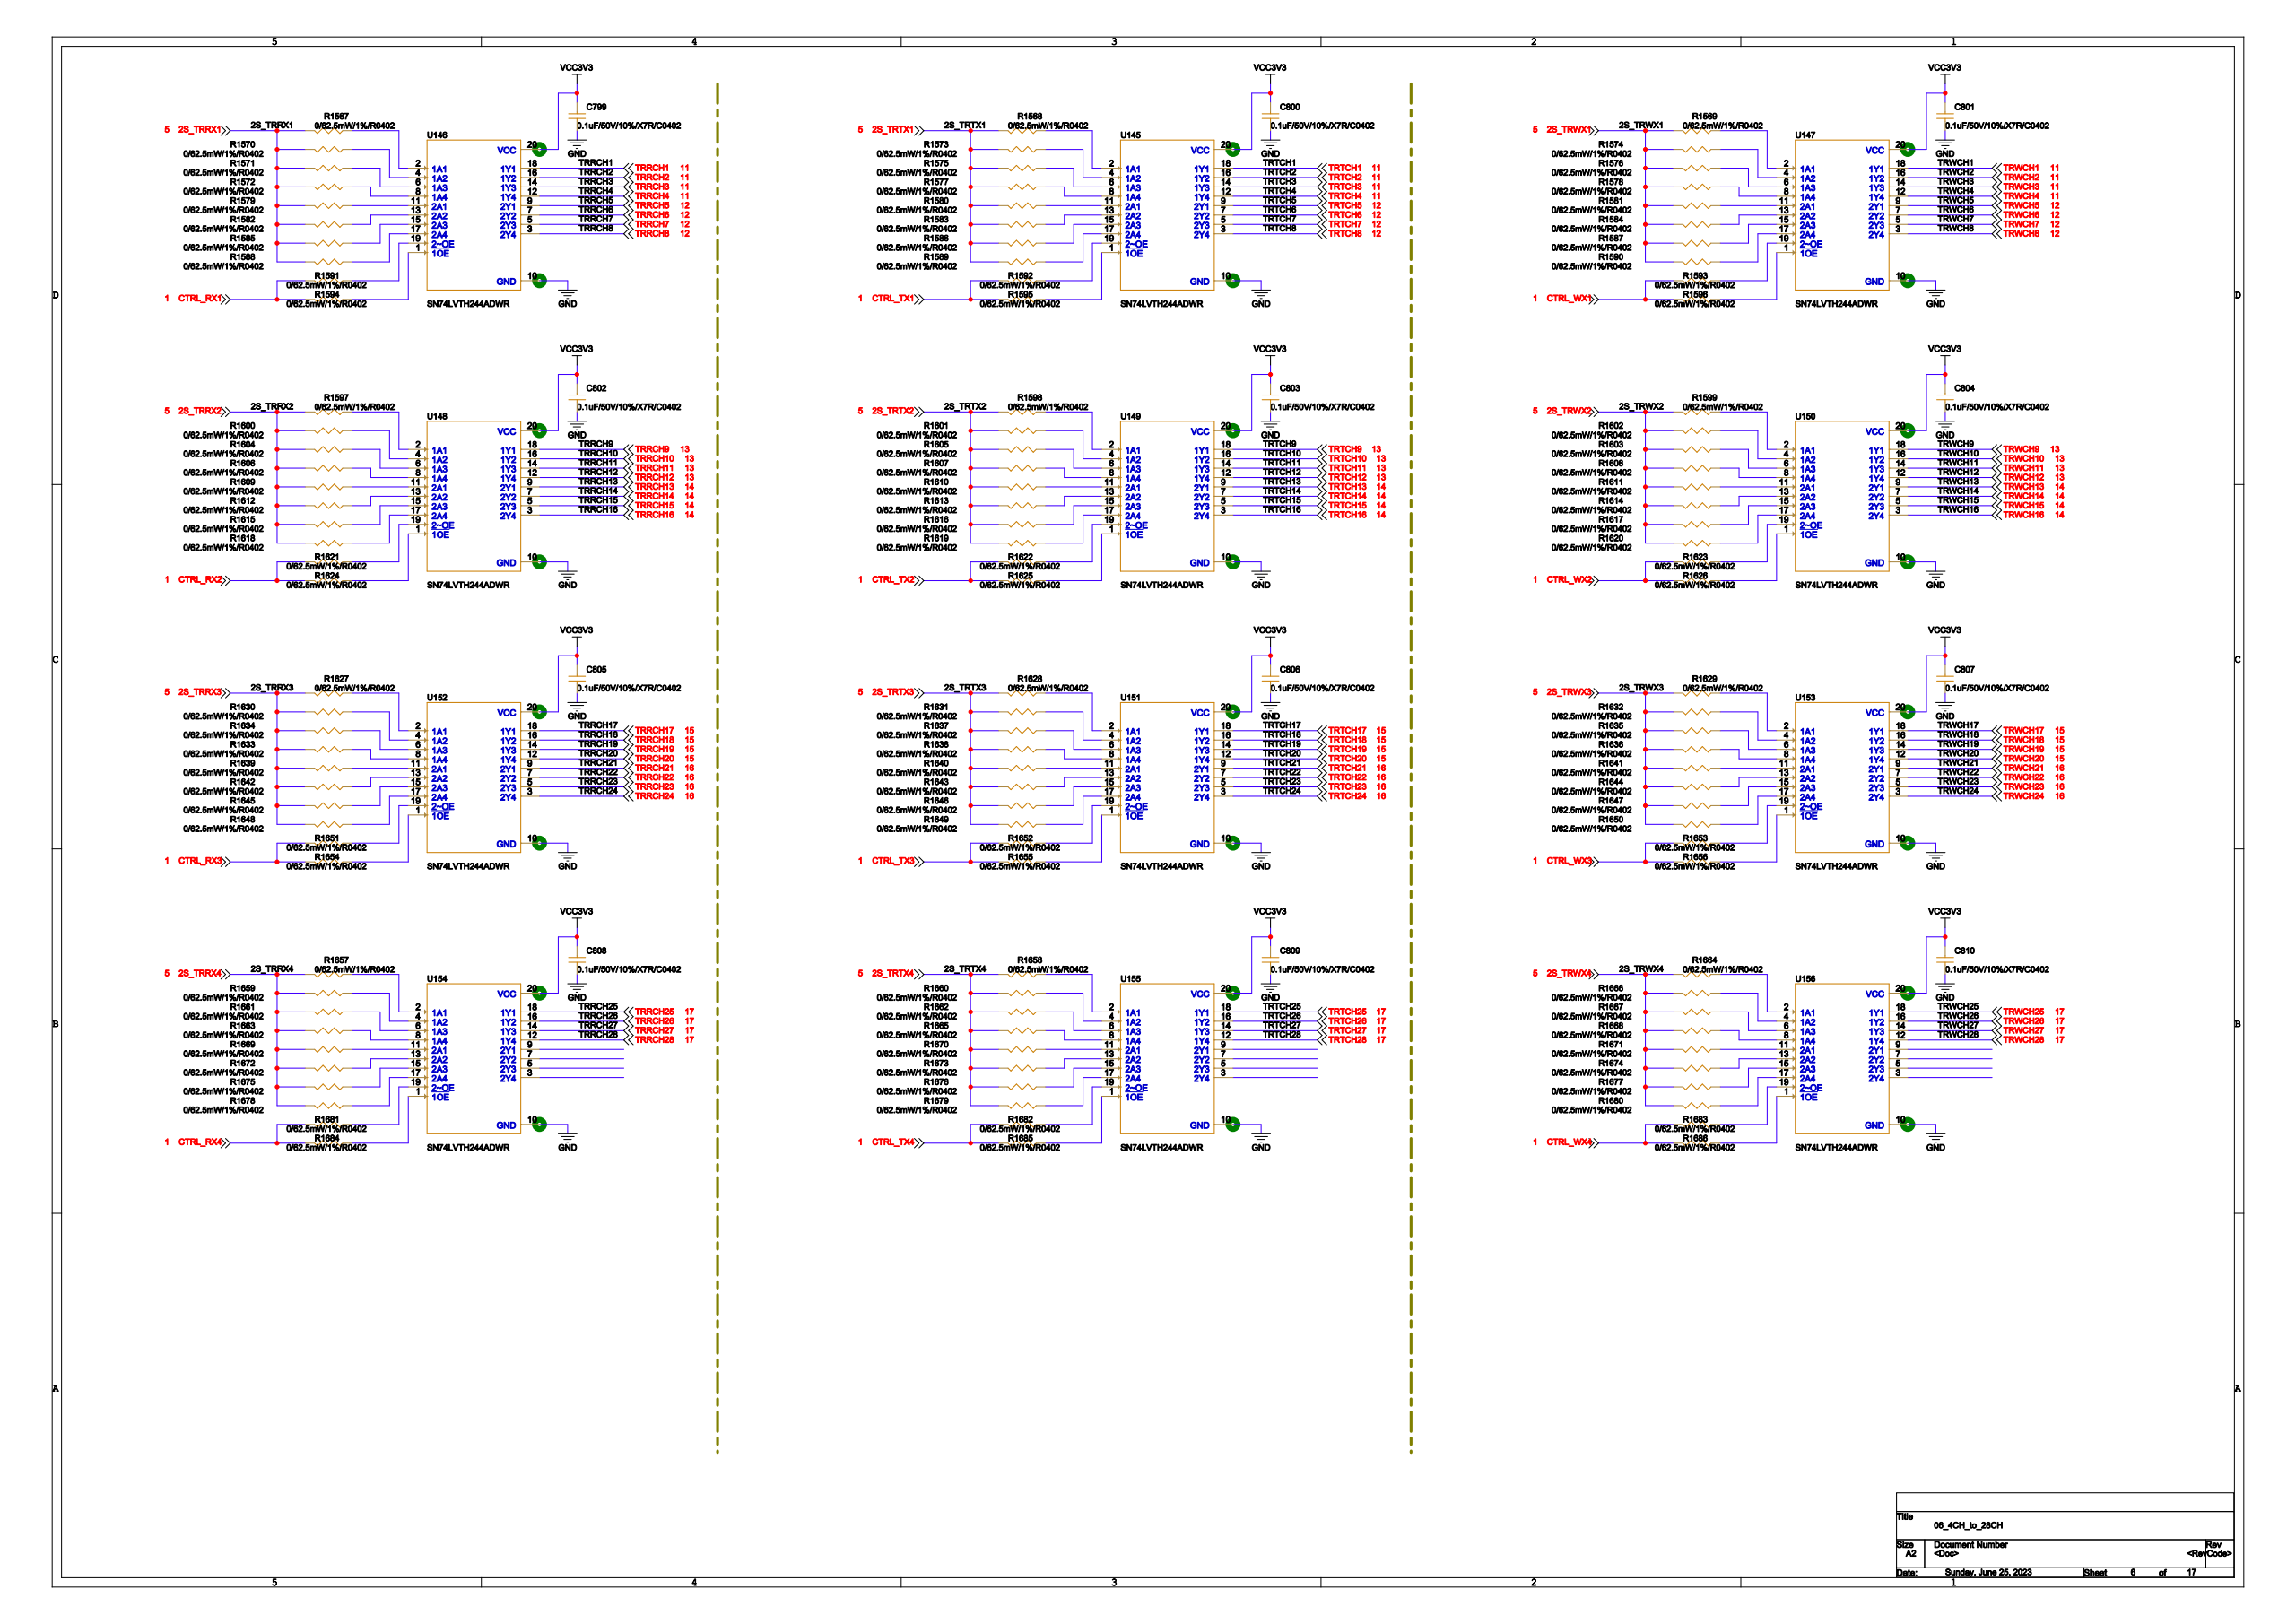Circuit board | Cadence Allegro | 1997 parts | 1536 nets | one sheet of the schematic
Parts on this sheet (reference | value | footprint):
C799 | 0.1uF/50V/10%/X7R/C0402 | 0402
C800 | 0.1uF/50V/10%/X7R/C0402 | 0402
C801 | 0.1uF/50V/10%/X7R/C0402 | 0402
C802 | 0.1uF/50V/10%/X7R/C0402 | 0402
C803 | 0.1uF/50V/10%/X7R/C0402 | 0402
C804 | 0.1uF/50V/10%/X7R/C0402 | 0402
C805 | 0.1uF/50V/10%/X7R/C0402 | 0402
C806 | 0.1uF/50V/10%/X7R/C0402 | 0402
C807 | 0.1uF/50V/10%/X7R/C0402 | 0402
C808 | 0.1uF/50V/10%/X7R/C0402 | 0402
C809 | 0.1uF/50V/10%/X7R/C0402 | 0402
C810 | 0.1uF/50V/10%/X7R/C0402 | 0402
R1567 | 0/62.5mW/1%/R0402 | 0402
R1568 | 0/62.5mW/1%/R0402 | 0402
R1569 | 0/62.5mW/1%/R0402 | 0402
R1570 | 0/62.5mW/1%/R0402 | 0402
R1571 | 0/62.5mW/1%/R0402 | 0402
R1572 | 0/62.5mW/1%/R0402 | 0402
R1573 | 0/62.5mW/1%/R0402 | 0402
R1574 | 0/62.5mW/1%/R0402 | 0402
R1575 | 0/62.5mW/1%/R0402 | 0402
R1576 | 0/62.5mW/1%/R0402 | 0402
R1577 | 0/62.5mW/1%/R0402 | 0402
R1578 | 0/62.5mW/1%/R0402 | 0402
R1579 | 0/62.5mW/1%/R0402 | 0402
R1580 | 0/62.5mW/1%/R0402 | 0402
R1581 | 0/62.5mW/1%/R0402 | 0402
R1582 | 0/62.5mW/1%/R0402 | 0402
R1583 | 0/62.5mW/1%/R0402 | 0402
R1584 | 0/62.5mW/1%/R0402 | 0402
R1585 | 0/62.5mW/1%/R0402 | 0402
R1586 | 0/62.5mW/1%/R0402 | 0402
R1587 | 0/62.5mW/1%/R0402 | 0402
R1588 | 0/62.5mW/1%/R0402 | 0402
R1589 | 0/62.5mW/1%/R0402 | 0402
R1590 | 0/62.5mW/1%/R0402 | 0402
R1591 | 0/62.5mW/1%/R0402 | 0402
R1592 | 0/62.5mW/1%/R0402 | 0402
R1593 | 0/62.5mW/1%/R0402 | 0402
R1594 | 0/62.5mW/1%/R0402 | 0402
R1595 | 0/62.5mW/1%/R0402 | 0402
R1596 | 0/62.5mW/1%/R0402 | 0402
R1597 | 0/62.5mW/1%/R0402 | 0402
R1598 | 0/62.5mW/1%/R0402 | 0402
R1599 | 0/62.5mW/1%/R0402 | 0402
R1600 | 0/62.5mW/1%/R0402 | 0402
R1601 | 0/62.5mW/1%/R0402 | 0402
R1602 | 0/62.5mW/1%/R0402 | 0402
R1603 | 0/62.5mW/1%/R0402 | 0402
R1604 | 0/62.5mW/1%/R0402 | 0402
R1605 | 0/62.5mW/1%/R0402 | 0402
R1606 | 0/62.5mW/1%/R0402 | 0402
R1607 | 0/62.5mW/1%/R0402 | 0402
R1608 | 0/62.5mW/1%/R0402 | 0402
R1609 | 0/62.5mW/1%/R0402 | 0402
R1610 | 0/62.5mW/1%/R0402 | 0402
R1611 | 0/62.5mW/1%/R0402 | 0402
R1612 | 0/62.5mW/1%/R0402 | 0402
R1613 | 0/62.5mW/1%/R0402 | 0402
R1614 | 0/62.5mW/1%/R0402 | 0402
R1615 | 0/62.5mW/1%/R0402 | 0402
R1616 | 0/62.5mW/1%/R0402 | 0402
R1617 | 0/62.5mW/1%/R0402 | 0402
R1618 | 0/62.5mW/1%/R0402 | 0402
R1619 | 0/62.5mW/1%/R0402 | 0402
R1620 | 0/62.5mW/1%/R0402 | 0402
R1621 | 0/62.5mW/1%/R0402 | 0402
R1622 | 0/62.5mW/1%/R0402 | 0402
R1623 | 0/62.5mW/1%/R0402 | 0402
R1624 | 0/62.5mW/1%/R0402 | 0402
R1625 | 0/62.5mW/1%/R0402 | 0402
R1626 | 0/62.5mW/1%/R0402 | 0402
R1627 | 0/62.5mW/1%/R0402 | 0402
R1628 | 0/62.5mW/1%/R0402 | 0402
R1629 | 0/62.5mW/1%/R0402 | 0402
R1630 | 0/62.5mW/1%/R0402 | 0402
R1631 | 0/62.5mW/1%/R0402 | 0402
R1632 | 0/62.5mW/1%/R0402 | 0402
R1633 | 0/62.5mW/1%/R0402 | 0402
R1634 | 0/62.5mW/1%/R0402 | 0402
R1635 | 0/62.5mW/1%/R0402 | 0402
R1636 | 0/62.5mW/1%/R0402 | 0402
R1637 | 0/62.5mW/1%/R0402 | 0402
R1638 | 0/62.5mW/1%/R0402 | 0402
R1639 | 0/62.5mW/1%/R0402 | 0402
R1640 | 0/62.5mW/1%/R0402 | 0402
R1641 | 0/62.5mW/1%/R0402 | 0402
R1642 | 0/62.5mW/1%/R0402 | 0402
R1643 | 0/62.5mW/1%/R0402 | 0402
R1644 | 0/62.5mW/1%/R0402 | 0402
R1645 | 0/62.5mW/1%/R0402 | 0402
R1646 | 0/62.5mW/1%/R0402 | 0402
R1647 | 0/62.5mW/1%/R0402 | 0402
R1648 | 0/62.5mW/1%/R0402 | 0402
R1649 | 0/62.5mW/1%/R0402 | 0402
R1650 | 0/62.5mW/1%/R0402 | 0402
R1651 | 0/62.5mW/1%/R0402 | 0402
R1652 | 0/62.5mW/1%/R0402 | 0402
R1653 | 0/62.5mW/1%/R0402 | 0402
R1654 | 0/62.5mW/1%/R0402 | 0402
R1655 | 0/62.5mW/1%/R0402 | 0402
R1656 | 0/62.5mW/1%/R0402 | 0402
R1657 | 0/62.5mW/1%/R0402 | 0402
R1658 | 0/62.5mW/1%/R0402 | 0402
R1659 | 0/62.5mW/1%/R0402 | 0402
R1660 | 0/62.5mW/1%/R0402 | 0402
R1661 | 0/62.5mW/1%/R0402 | 0402
R1662 | 0/62.5mW/1%/R0402 | 0402
R1663 | 0/62.5mW/1%/R0402 | 0402
R1664 | 0/62.5mW/1%/R0402 | 0402
R1665 | 0/62.5mW/1%/R0402 | 0402
R1666 | 0/62.5mW/1%/R0402 | 0402
R1667 | 0/62.5mW/1%/R0402 | 0402
R1668 | 0/62.5mW/1%/R0402 | 0402
R1669 | 0/62.5mW/1%/R0402 | 0402
R1670 | 0/62.5mW/1%/R0402 | 0402
R1671 | 0/62.5mW/1%/R0402 | 0402
R1672 | 0/62.5mW/1%/R0402 | 0402
R1673 | 0/62.5mW/1%/R0402 | 0402
R1674 | 0/62.5mW/1%/R0402 | 0402
R1675 | 0/62.5mW/1%/R0402 | 0402
R1676 | 0/62.5mW/1%/R0402 | 0402
R1677 | 0/62.5mW/1%/R0402 | 0402
R1678 | 0/62.5mW/1%/R0402 | 0402
R1679 | 0/62.5mW/1%/R0402 | 0402
R1680 | 0/62.5mW/1%/R0402 | 0402
R1681 | 0/62.5mW/1%/R0402 | 0402
R1682 | 0/62.5mW/1%/R0402 | 0402
R1683 | 0/62.5mW/1%/R0402 | 0402
R1684 | 0/62.5mW/1%/R0402 | 0402
R1685 | 0/62.5mW/1%/R0402 | 0402
R1686 | 0/62.5mW/1%/R0402 | 0402
U145 | SN74LVTH244ADWR | SOIC127P1030X265-20N
U146 | SN74LVTH244ADWR | SOIC127P1030X265-20N
U147 | SN74LVTH244ADWR | SOIC127P1030X265-20N
U148 | SN74LVTH244ADWR | SOIC127P1030X265-20N
U149 | SN74LVTH244ADWR | SOIC127P1030X265-20N
U150 | SN74LVTH244ADWR | SOIC127P1030X265-20N
U151 | SN74LVTH244ADWR | SOIC127P1030X265-20N
U152 | SN74LVTH244ADWR | SOIC127P1030X265-20N
U153 | SN74LVTH244ADWR | SOIC127P1030X265-20N
U154 | SN74LVTH244ADWR | SOIC127P1030X265-20N
U155 | SN74LVTH244ADWR | SOIC127P1030X265-20N
U156 | SN74LVTH244ADWR | SOIC127P1030X265-20N
Nets of these parts (net: part-pin ...):
3.3V: C799-1 C800-1 C801-1 C802-1 C803-1 C804-1 C805-1 C806-1 C807-1 C808-1 C809-1 C810-1 U145-20 U146-20 U147-20 U148-20 U149-20 U150-20 U151-20 U152-20 U153-20 U154-20 U155-20 U156-20
AGND: C799-2 C800-2 C801-2 C802-2 C803-2 C804-2 C805-2 C806-2 C807-2 C808-2 C809-2 C810-2 U145-10 U146-10 U147-10 U148-10 U149-10 U150-10 U151-10 U152-10 U153-10 U154-10 U155-10 U156-10
CTRL_RX3: R1651-1 R1654-1
CTRL_RX2: R1621-1 R1624-1
CTRL_WX2: R1623-1 R1626-1
CTRL_TX2: R1622-1 R1625-1
CTRL_TX1: R1592-1 R1595-1
CTRL_WX4: R1683-1 R1686-1
CTRL_RX1: R1591-1 R1594-1
CTRL_WX1: R1593-1 R1596-1
CTRL_RX4: R1681-1 R1684-1
CTRL_TX4: R1682-1 R1685-1
CTRL_WX3: R1653-1 R1656-1
CTRL_TX3: R1652-1 R1655-1
2S_TRRX1: R1567-1 R1570-1 R1571-1 R1572-1 R1579-1 R1582-1 R1585-1 R1588-1
N23955636: R1567-2 U146-2
2S_TRTX1: R1568-1 R1573-1 R1575-1 R1577-1 R1580-1 R1583-1 R1586-1 R1589-1
N23963258: R1568-2 U145-2
2S_TRWX1: R1569-1 R1574-1 R1576-1 R1578-1 R1581-1 R1584-1 R1587-1 R1590-1
N23976669: R1569-2 U147-2
N23955843: R1570-2 U146-4
N23955864: R1571-2 U146-6
N23955873: R1572-2 U146-8
N23963345: R1573-2 U145-4
N23976782: R1574-2 U147-4
N23963355: R1575-2 U145-6
N23976792: R1576-2 U147-6
N23963361: R1577-2 U145-8
N23976798: R1578-2 U147-8
N23955883: R1579-2 U146-11
N23963367: R1580-2 U145-11
N23976804: R1581-2 U147-11
N23955886: R1582-2 U146-13
N23963369: R1583-2 U145-13
N23976806: R1584-2 U147-13
N23955895: R1585-2 U146-15
N23963375: R1586-2 U145-15
N23976812: R1587-2 U147-15
N23955904: R1588-2 U146-17
N23963381: R1589-2 U145-17
N23976818: R1590-2 U147-17
N23955981: R1591-2 U146-19
N23963403: R1592-2 U145-19
N23976840: R1593-2 U147-19
N23955993: R1594-2 U146-1
N23963409: R1595-2 U145-1
N23976846: R1596-2 U147-1
2S_TRRX2: R1597-1 R1600-1 R1604-1 R1606-1 R1609-1 R1612-1 R1615-1 R1618-1
N23957290: R1597-2 U148-2
2S_TRTX2: R1598-1 R1601-1 R1605-1 R1607-1 R1610-1 R1613-1 R1616-1 R1619-1
N23963537: R1598-2 U149-2
2S_TRWX2: R1599-1 R1602-1 R1603-1 R1608-1 R1611-1 R1614-1 R1617-1 R1620-1
N23976942: R1599-2 U150-2
N23957377: R1600-2 U148-4
N23963650: R1601-2 U149-4
N23977055: R1602-2 U150-4
N23977065: R1603-2 U150-6
N23957387: R1604-2 U148-6
N23963660: R1605-2 U149-6
N23957393: R1606-2 U148-8
N23963666: R1607-2 U149-8
N23977071: R1608-2 U150-8
N23957399: R1609-2 U148-11
N23963672: R1610-2 U149-11
N23977077: R1611-2 U150-11
N23957401: R1612-2 U148-13
N23963674: R1613-2 U149-13
N23977079: R1614-2 U150-13
N23957407: R1615-2 U148-15
N23963680: R1616-2 U149-15
N23977085: R1617-2 U150-15
N23957413: R1618-2 U148-17
N23963686: R1619-2 U149-17
N23977091: R1620-2 U150-17
N23957435: R1621-2 U148-19
N23963708: R1622-2 U149-19
N23977113: R1623-2 U150-19
N23957441: R1624-2 U148-1
N23963714: R1625-2 U149-1
N23977119: R1626-2 U150-1
2S_TRRX3: R1627-1 R1630-1 R1633-1 R1634-1 R1639-1 R1642-1 R1645-1 R1648-1
N23958041: R1627-2 U152-2
2S_TRTX3: R1628-1 R1631-1 R1637-1 R1638-1 R1640-1 R1643-1 R1646-1 R1649-1
N23963810: R1628-2 U151-2
2S_TRWX3: R1629-1 R1632-1 R1635-1 R1636-1 R1641-1 R1644-1 R1647-1 R1650-1
N23977215: R1629-2 U153-2
N23958128: R1630-2 U152-4
N23963923: R1631-2 U151-4
N23977328: R1632-2 U153-4
N23958144: R1633-2 U152-8
N23958138: R1634-2 U152-6
N23977338: R1635-2 U153-6
N23977344: R1636-2 U153-8
N23963933: R1637-2 U151-6
N23963939: R1638-2 U151-8
N23958150: R1639-2 U152-11
N23963945: R1640-2 U151-11
N23977350: R1641-2 U153-11
N23958152: R1642-2 U152-13
N23963947: R1643-2 U151-13
N23977352: R1644-2 U153-13
N23958158: R1645-2 U152-15
N23963953: R1646-2 U151-15
N23977358: R1647-2 U153-15
N23958164: R1648-2 U152-17
N23963959: R1649-2 U151-17
N23977364: R1650-2 U153-17
N23958186: R1651-2 U152-19
N23963981: R1652-2 U151-19
N23977386: R1653-2 U153-19
N23958192: R1654-2 U152-1
N23963987: R1655-2 U151-1
N23977392: R1656-2 U153-1
2S_TRRX4: R1657-1 R1659-1 R1661-1 R1663-1 R1669-1 R1672-1 R1675-1 R1678-1
N23958837: R1657-2 U154-2
2S_TRTX4: R1658-1 R1660-1 R1662-1 R1665-1 R1670-1 R1673-1 R1676-1 R1679-1
N23964083: R1658-2 U155-2
N23958924: R1659-2 U154-4
N23964196: R1660-2 U155-4
N23958934: R1661-2 U154-6
N23964206: R1662-2 U155-6
N23958940: R1663-2 U154-8
2S_TRWX4: R1664-1 R1666-1 R1667-1 R1668-1 R1671-1 R1674-1 R1677-1 R1680-1
N23977488: R1664-2 U156-2
N23964212: R1665-2 U155-8
N23977601: R1666-2 U156-4
N23977611: R1667-2 U156-6
N23977617: R1668-2 U156-8
N23958946: R1669-2 U154-11
N23964218: R1670-2 U155-11
N23977623: R1671-2 U156-11
N23958948: R1672-2 U154-13
N23964220: R1673-2 U155-13
N23977625: R1674-2 U156-13
N23958954: R1675-2 U154-15
N23964226: R1676-2 U155-15
N23977631: R1677-2 U156-15
N23958960: R1678-2 U154-17
N23964232: R1679-2 U155-17
N23977637: R1680-2 U156-17
N23958982: R1681-2 U154-19
N23964254: R1682-2 U155-19
N23977659: R1683-2 U156-19
N23958988: R1684-2 U154-1
N23964260: R1685-2 U155-1
N23977665: R1686-2 U156-1
TRRCH1: U146-18
TRTCH1: U145-18
TRWCH1: U147-18
TRRCH2: U146-16
TRTCH2: U145-16
TRWCH2: U147-16
TRRCH3: U146-14
TRTCH3: U145-14
TRWCH3: U147-14
TRRCH4: U146-12
TRTCH4: U145-12
TRWCH4: U147-12
TRRCH5: U146-9
TRTCH5: U145-9
TRWCH5: U147-9
TRRCH6: U146-7
TRTCH6: U145-7
TRWCH6: U147-7
TRTCH7: U145-5
TRRCH7: U146-5
TRWCH7: U147-5
TRRCH8: U146-3
TRTCH8: U145-3
TRWCH8: U147-3
TRRCH9: U148-18
TRTCH9: U149-18
TRWCH9: U150-18
TRRCH10: U148-16
TRTCH10: U149-16
TRWCH10: U150-16
TRRCH11: U148-14
TRTCH11: U149-14
TRWCH11: U150-14
TRRCH12: U148-12
TRTCH12: U149-12
TRWCH12: U150-12
TRRCH13: U148-9
TRTCH13: U149-9
TRWCH13: U150-9
TRTCH14: U149-7
TRRCH14: U148-7
TRWCH14: U150-7
TRTCH15: U149-5
TRWCH15: U150-5
TRRCH15: U148-5
TRRCH16: U148-3
TRTCH16: U149-3
TRWCH16: U150-3
TRRCH17: U152-18
TRTCH17: U151-18
TRWCH17: U153-18
TRRCH18: U152-16
TRTCH18: U151-16
TRWCH18: U153-16
TRRCH19: U152-14
TRTCH19: U151-14
TRWCH19: U153-14
TRRCH20: U152-12
TRTCH20: U151-12
TRWCH20: U153-12
TRRCH21: U152-9
TRTCH21: U151-9
TRWCH21: U153-9
TRRCH22: U152-7
TRTCH22: U151-7
TRWCH22: U153-7
TRRCH23: U152-5
TRTCH23: U151-5
TRWCH23: U153-5
TRRCH24: U152-3
TRTCH24: U151-3
TRWCH24: U153-3
TRRCH25: U154-18
TRTCH25: U155-18
TRWCH25: U156-18
TRRCH26: U154-16
TRTCH26: U155-16
TRWCH26: U156-16
TRRCH27: U154-14
TRTCH27: U155-14
TRWCH27: U156-14
TRRCH28: U154-12
TRWCH28: U156-12
TRTCH28: U155-12
N23959088: U154-9
N23959091: U154-7
N23959102: U154-5
N23959105: U154-3
N23964344: U155-9
N23964347: U155-7
N23964350: U155-5
N23964353: U155-3
N23977749: U156-9
N23977752: U156-7
N23977755: U156-5
N23977758: U156-3